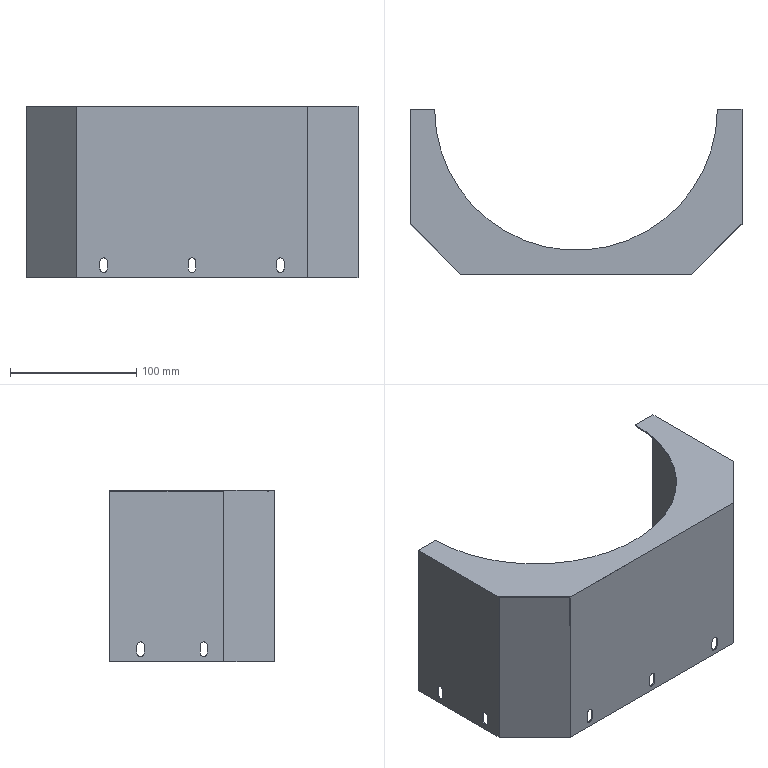Part | SolidWorks | features HoleWzd 2, Chamfer 1, Cut 1, Extrusion 1, Shell 1 | 1 solid | 51 faces | box 263 x 130.5 x 136 mm | volume 76891 mm3 | plane 29 | cylinder 22 | commonest cylinder face diameters 5.8 x21 224 x1